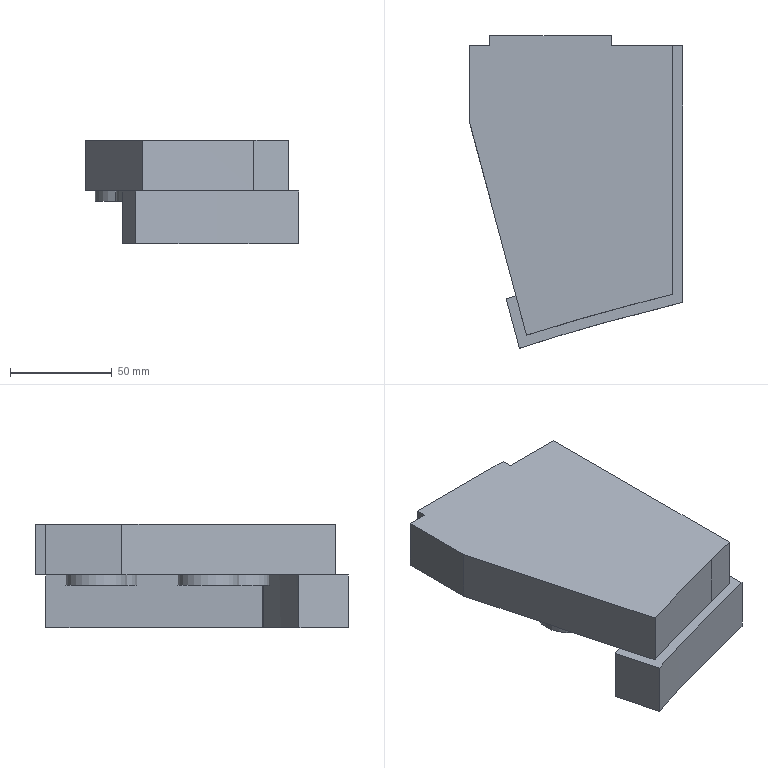Part | NX | features solid 2 | 1 solid | 29 faces | box 104.575 x 153.355 x 51 mm | volume 442885 mm3 | plane 20 | spline 5 | cylinder 4 | commonest cylinder face diameters 30 x4
STEP:
#1=CARTESIAN_POINT('',(-394.575,600.,45.));
#2=VERTEX_POINT('',#1);
#3=CARTESIAN_POINT('',(-394.575,600.,20.));
#4=VERTEX_POINT('',#3);
#5=CARTESIAN_POINT('',(-394.575,600.,50.));
#6=DIRECTION('',(0.,0.,-1.));
#7=VECTOR('',#6,1000.);
#8=LINE('',#5,#7);
#9=EDGE_CURVE('',#2,#4,#8,.T.);
#10=ORIENTED_EDGE('',*,*,#9,.F.);
#11=CARTESIAN_POINT('',(-384.575,600.,45.));
#12=VERTEX_POINT('',#11);
#13=CARTESIAN_POINT('',(-290.,600.,45.));
#14=DIRECTION('',(-1.,0.,0.));
#15=VECTOR('',#14,1000.);
#16=LINE('',#13,#15);
#17=EDGE_CURVE('',#12,#2,#16,.T.);
#18=ORIENTED_EDGE('',*,*,#17,.F.);
#19=CARTESIAN_POINT('',(-384.575,600.,20.));
#20=VERTEX_POINT('',#19);
#21=CARTESIAN_POINT('',(-384.575,600.,50.));
#22=DIRECTION('',(0.,0.,-1.));
#23=VECTOR('',#22,1000.);
#24=LINE('',#21,#23);
#25=EDGE_CURVE('',#12,#20,#24,.T.);
#26=ORIENTED_EDGE('',*,*,#25,.T.);
#27=CARTESIAN_POINT('',(-561.977,600.,20.));
#28=DIRECTION('',(1.,0.,0.));
#29=VECTOR('',#28,1000.);
#30=LINE('',#27,#29);
#31=EDGE_CURVE('',#20,#4,#30,.F.);
#32=ORIENTED_EDGE('',*,*,#31,.T.);
#33=EDGE_LOOP('',(#10,#18,#26,#32));
#34=FACE_BOUND('',#33,.T.);
#35=CARTESIAN_POINT('',(-290.,600.,50.));
#36=DIRECTION('',(0.,-1.,0.));
#37=DIRECTION('',(0.,0.,-1.));
#38=AXIS2_PLACEMENT_3D('',#35,#36,#37);
#39=PLANE('',#38);
#40=ADVANCED_FACE('',(#34),#39,.F.);
#41=ORIENTED_EDGE('',*,*,#17,.T.);
#42=CARTESIAN_POINT('',(-394.575,562.679,45.));
#43=VERTEX_POINT('',#42);
#44=CARTESIAN_POINT('',(-394.575,-794.984,45.));
#45=DIRECTION('',(0.,-1.,0.));
#46=VECTOR('',#45,1000.);
#47=LINE('',#44,#46);
#48=EDGE_CURVE('',#2,#43,#47,.T.);
#49=ORIENTED_EDGE('',*,*,#48,.T.);
#50=CARTESIAN_POINT('',(-366.532,458.021,45.));
#51=VERTEX_POINT('',#50);
#52=CARTESIAN_POINT('',(-371.65,477.121,45.));
#53=DIRECTION('',(-0.2588,0.9659,0.));
#54=VECTOR('',#53,1000.);
#55=LINE('',#52,#54);
#56=EDGE_CURVE('',#43,#51,#55,.F.);
#57=ORIENTED_EDGE('',*,*,#56,.T.);
#58=CARTESIAN_POINT('',(-311.881,473.776,45.));
#59=VERTEX_POINT('',#58);
#60=CARTESIAN_POINT('',(-366.532,458.021,45.));
#61=CARTESIAN_POINT('',(-361.995,459.474,45.));
#62=CARTESIAN_POINT('',(-355.189,461.6,45.));
#63=CARTESIAN_POINT('',(-347.268,463.978,45.));
#64=CARTESIAN_POINT('',(-343.294,465.147,45.));
#65=CARTESIAN_POINT('',(-341.047,465.801,45.));
#66=CARTESIAN_POINT('',(-339.295,466.308,45.));
#67=CARTESIAN_POINT('',(-337.801,466.736,45.));
#68=CARTESIAN_POINT('',(-335.683,467.34,45.));
#69=CARTESIAN_POINT('',(-331.945,468.393,45.));
#70=CARTESIAN_POINT('',(-326.364,469.934,45.));
#71=CARTESIAN_POINT('',(-319.327,471.827,45.));
#72=CARTESIAN_POINT('',(-314.402,473.121,45.));
#73=CARTESIAN_POINT('',(-311.881,473.776,45.));
#74=B_SPLINE_CURVE_WITH_KNOTS('',3,(#60,#61,#62,#63,#64,#65,#66,#67,#68,#69,#70,#71,#72,#73),.UNSPECIFIED.,.F.,.F.,(4,1,1,1,1,1,1,1,1,1,1,4),(0.,0.25,0.375,0.4375,0.4688,0.5,0.5312,0.5625,0.625,0.75,0.875,1.),.UNSPECIFIED.);
#75=EDGE_CURVE('',#51,#59,#74,.T.);
#76=ORIENTED_EDGE('',*,*,#75,.T.);
#77=CARTESIAN_POINT('',(-295.,478.098,45.));
#78=VERTEX_POINT('',#77);
#79=CARTESIAN_POINT('',(-311.881,473.776,45.));
#80=CARTESIAN_POINT('',(-307.372,474.947,45.));
#81=CARTESIAN_POINT('',(-301.745,476.387,45.));
#82=CARTESIAN_POINT('',(-295.,478.098,45.));
#83=B_SPLINE_CURVE_WITH_KNOTS('',3,(#79,#80,#81,#82),.UNSPECIFIED.,.F.,.F.,(4,4),(0.,1.),.UNSPECIFIED.);
#84=EDGE_CURVE('',#59,#78,#83,.T.);
#85=ORIENTED_EDGE('',*,*,#84,.T.);
#86=CARTESIAN_POINT('',(-295.,600.,45.));
#87=VERTEX_POINT('',#86);
#88=CARTESIAN_POINT('',(-295.,-794.984,45.));
#89=DIRECTION('',(0.,1.,0.));
#90=VECTOR('',#89,1000.);
#91=LINE('',#88,#90);
#92=EDGE_CURVE('',#78,#87,#91,.T.);
#93=ORIENTED_EDGE('',*,*,#92,.T.);
#94=CARTESIAN_POINT('',(-325.,600.,45.));
#95=VERTEX_POINT('',#94);
#96=CARTESIAN_POINT('',(-290.,600.,45.));
#97=DIRECTION('',(-1.,0.,0.));
#98=VECTOR('',#97,1000.);
#99=LINE('',#96,#98);
#100=EDGE_CURVE('',#87,#95,#99,.T.);
#101=ORIENTED_EDGE('',*,*,#100,.T.);
#102=CARTESIAN_POINT('',(-325.,605.,45.));
#103=VERTEX_POINT('',#102);
#104=CARTESIAN_POINT('',(-325.,605.,45.));
#105=DIRECTION('',(0.,-1.,0.));
#106=VECTOR('',#105,1000.);
#107=LINE('',#104,#106);
#108=EDGE_CURVE('',#103,#95,#107,.T.);
#109=ORIENTED_EDGE('',*,*,#108,.F.);
#110=CARTESIAN_POINT('',(-384.575,605.,45.));
#111=VERTEX_POINT('',#110);
#112=CARTESIAN_POINT('',(-290.,605.,45.));
#113=DIRECTION('',(-1.,0.,0.));
#114=VECTOR('',#113,1000.);
#115=LINE('',#112,#114);
#116=EDGE_CURVE('',#103,#111,#115,.T.);
#117=ORIENTED_EDGE('',*,*,#116,.T.);
#118=CARTESIAN_POINT('',(-384.575,605.,45.));
#119=DIRECTION('',(0.,-1.,0.));
#120=VECTOR('',#119,1000.);
#121=LINE('',#118,#120);
#122=EDGE_CURVE('',#111,#12,#121,.T.);
#123=ORIENTED_EDGE('',*,*,#122,.T.);
#124=EDGE_LOOP('',(#41,#49,#57,#76,#85,#93,#101,#109,#117,#123));
#125=FACE_BOUND('',#124,.T.);
#126=CARTESIAN_POINT('',(-80.139,-794.984,45.));
#127=DIRECTION('',(0.,0.,1.));
#128=DIRECTION('',(1.,0.,0.));
#129=AXIS2_PLACEMENT_3D('',#126,#127,#128);
#130=PLANE('',#129);
#131=ADVANCED_FACE('',(#125),#130,.T.);
#132=CARTESIAN_POINT('',(-354.757,570.324,20.));
#133=VERTEX_POINT('',#132);
#134=CARTESIAN_POINT('',(-339.757,570.324,20.));
#135=DIRECTION('',(0.,0.,-1.));
#136=DIRECTION('',(-1.,0.,0.));
#137=AXIS2_PLACEMENT_3D('',#134,#135,#136);
#138=CIRCLE('',#137,15.);
#139=EDGE_CURVE('',#133,#133,#138,.F.);
#140=ORIENTED_EDGE('',*,*,#139,.T.);
#141=EDGE_LOOP('',(#140));
#142=FACE_BOUND('',#141,.T.);
#143=CARTESIAN_POINT('',(-389.757,575.324,20.));
#144=VERTEX_POINT('',#143);
#145=CARTESIAN_POINT('',(-374.757,575.324,20.));
#146=DIRECTION('',(0.,0.,-1.));
#147=DIRECTION('',(-1.,0.,0.));
#148=AXIS2_PLACEMENT_3D('',#145,#146,#147);
#149=CIRCLE('',#148,15.);
#150=EDGE_CURVE('',#144,#144,#149,.F.);
#151=ORIENTED_EDGE('',*,*,#150,.T.);
#152=EDGE_LOOP('',(#151));
#153=FACE_BOUND('',#152,.T.);
#154=CARTESIAN_POINT('',(-349.757,505.324,20.));
#155=VERTEX_POINT('',#154);
#156=CARTESIAN_POINT('',(-334.757,505.324,20.));
#157=DIRECTION('',(0.,0.,-1.));
#158=DIRECTION('',(-1.,0.,0.));
#159=AXIS2_PLACEMENT_3D('',#156,#157,#158);
#160=CIRCLE('',#159,15.);
#161=EDGE_CURVE('',#155,#155,#160,.F.);
#162=ORIENTED_EDGE('',*,*,#161,.T.);
#163=EDGE_LOOP('',(#162));
#164=FACE_BOUND('',#163,.T.);
#165=CARTESIAN_POINT('',(-379.757,520.324,20.));
#166=VERTEX_POINT('',#165);
#167=CARTESIAN_POINT('',(-364.757,520.324,20.));
#168=DIRECTION('',(0.,0.,-1.));
#169=DIRECTION('',(-1.,0.,0.));
#170=AXIS2_PLACEMENT_3D('',#167,#168,#169);
#171=CIRCLE('',#170,15.);
#172=EDGE_CURVE('',#166,#166,#171,.F.);
#173=ORIENTED_EDGE('',*,*,#172,.T.);
#174=EDGE_LOOP('',(#173));
#175=FACE_BOUND('',#174,.T.);
#176=CARTESIAN_POINT('',(-394.575,562.679,20.));
#177=VERTEX_POINT('',#176);
#178=CARTESIAN_POINT('',(-394.575,359.461,20.));
#179=DIRECTION('',(0.,1.,0.));
#180=VECTOR('',#179,1000.);
#181=LINE('',#178,#180);
#182=EDGE_CURVE('',#4,#177,#181,.F.);
#183=ORIENTED_EDGE('',*,*,#182,.F.);
#184=ORIENTED_EDGE('',*,*,#31,.F.);
#185=CARTESIAN_POINT('',(-384.575,605.,20.));
#186=VERTEX_POINT('',#185);
#187=CARTESIAN_POINT('',(-384.575,605.,20.));
#188=DIRECTION('',(0.,-1.,0.));
#189=VECTOR('',#188,1000.);
#190=LINE('',#187,#189);
#191=EDGE_CURVE('',#186,#20,#190,.T.);
#192=ORIENTED_EDGE('',*,*,#191,.F.);
#193=CARTESIAN_POINT('',(-325.,605.,20.));
#194=VERTEX_POINT('',#193);
#195=CARTESIAN_POINT('',(-561.977,605.,20.));
#196=DIRECTION('',(1.,0.,0.));
#197=VECTOR('',#196,1000.);
#198=LINE('',#195,#197);
#199=EDGE_CURVE('',#194,#186,#198,.F.);
#200=ORIENTED_EDGE('',*,*,#199,.F.);
#201=CARTESIAN_POINT('',(-325.,600.,20.));
#202=VERTEX_POINT('',#201);
#203=CARTESIAN_POINT('',(-325.,605.,20.));
#204=DIRECTION('',(0.,-1.,0.));
#205=VECTOR('',#204,1000.);
#206=LINE('',#203,#205);
#207=EDGE_CURVE('',#194,#202,#206,.T.);
#208=ORIENTED_EDGE('',*,*,#207,.T.);
#209=CARTESIAN_POINT('',(-315.,600.,20.));
#210=VERTEX_POINT('',#209);
#211=CARTESIAN_POINT('',(-561.977,600.,20.));
#212=DIRECTION('',(1.,0.,0.));
#213=VECTOR('',#212,1000.);
#214=LINE('',#211,#213);
#215=EDGE_CURVE('',#210,#202,#214,.F.);
#216=ORIENTED_EDGE('',*,*,#215,.F.);
#217=CARTESIAN_POINT('',(-315.,493.628,20.));
#218=VERTEX_POINT('',#217);
#219=CARTESIAN_POINT('',(-315.,359.461,20.));
#220=DIRECTION('',(0.,1.,0.));
#221=VECTOR('',#220,1000.);
#222=LINE('',#219,#221);
#223=EDGE_CURVE('',#210,#218,#222,.F.);
#224=ORIENTED_EDGE('',*,*,#223,.T.);
#225=CARTESIAN_POINT('',(-316.72,493.182,20.));
#226=VERTEX_POINT('',#225);
#227=CARTESIAN_POINT('',(-316.72,493.182,20.));
#228=CARTESIAN_POINT('',(-316.146,493.331,20.));
#229=CARTESIAN_POINT('',(-315.573,493.48,20.));
#230=CARTESIAN_POINT('',(-315.,493.628,20.));
#231=B_SPLINE_CURVE_WITH_KNOTS('',3,(#227,#228,#229,#230),.UNSPECIFIED.,.F.,.F.,(4,4),(0.4269,0.4287),.UNSPECIFIED.);
#232=EDGE_CURVE('',#226,#218,#231,.T.);
#233=ORIENTED_EDGE('',*,*,#232,.F.);
#234=CARTESIAN_POINT('',(-371.714,477.362,20.));
#235=VERTEX_POINT('',#234);
#236=CARTESIAN_POINT('',(-371.714,477.362,20.));
#237=CARTESIAN_POINT('',(-353.545,483.162,20.));
#238=CARTESIAN_POINT('',(-335.183,488.388,20.));
#239=CARTESIAN_POINT('',(-316.72,493.182,20.));
#240=B_SPLINE_CURVE_WITH_KNOTS('',3,(#236,#237,#238,#239),.UNSPECIFIED.,.F.,.F.,(4,4),(0.6725,0.7298),.UNSPECIFIED.);
#241=EDGE_CURVE('',#235,#226,#240,.T.);
#242=ORIENTED_EDGE('',*,*,#241,.F.);
#243=CARTESIAN_POINT('',(-371.65,477.121,20.));
#244=DIRECTION('',(0.2588,-0.9659,0.));
#245=VECTOR('',#244,1000.);
#246=LINE('',#243,#245);
#247=EDGE_CURVE('',#177,#235,#246,.T.);
#248=ORIENTED_EDGE('',*,*,#247,.F.);
#249=EDGE_LOOP('',(#183,#184,#192,#200,#208,#216,#224,#233,#242,#248));
#250=FACE_BOUND('',#249,.T.);
#251=CARTESIAN_POINT('',(-561.977,359.461,20.));
#252=DIRECTION('',(0.,0.,-1.));
#253=DIRECTION('',(-1.,0.,0.));
#254=AXIS2_PLACEMENT_3D('',#251,#252,#253);
#255=PLANE('',#254);
#256=ADVANCED_FACE('',(#142,#153,#164,#175,#250),#255,.T.);
#257=ORIENTED_EDGE('',*,*,#56,.F.);
#258=CARTESIAN_POINT('',(-394.575,562.679,20.));
#259=DIRECTION('',(0.,0.,-1.));
#260=VECTOR('',#259,1000.);
#261=LINE('',#258,#260);
#262=EDGE_CURVE('',#43,#177,#261,.T.);
#263=ORIENTED_EDGE('',*,*,#262,.T.);
#264=ORIENTED_EDGE('',*,*,#247,.T.);
#265=CARTESIAN_POINT('',(-366.532,458.021,20.));
#266=VERTEX_POINT('',#265);
#267=CARTESIAN_POINT('',(-371.65,477.121,20.));
#268=DIRECTION('',(0.2588,-0.9659,0.));
#269=VECTOR('',#268,1000.);
#270=LINE('',#267,#269);
#271=EDGE_CURVE('',#235,#266,#270,.T.);
#272=ORIENTED_EDGE('',*,*,#271,.T.);
#273=CARTESIAN_POINT('',(-366.532,458.021,32.5));
#274=DIRECTION('',(0.,0.,-1.));
#275=VECTOR('',#274,1000.);
#276=LINE('',#273,#275);
#277=EDGE_CURVE('',#266,#51,#276,.F.);
#278=ORIENTED_EDGE('',*,*,#277,.T.);
#279=EDGE_LOOP('',(#257,#263,#264,#272,#278));
#280=FACE_BOUND('',#279,.T.);
#281=CARTESIAN_POINT('',(-371.65,477.121,20.));
#282=DIRECTION('',(-0.9659,-0.2588,0.));
#283=DIRECTION('',(0.2588,-0.9659,0.));
#284=AXIS2_PLACEMENT_3D('',#281,#282,#283);
#285=PLANE('',#284);
#286=ADVANCED_FACE('',(#280),#285,.T.);
#287=ORIENTED_EDGE('',*,*,#277,.F.);
#288=CARTESIAN_POINT('',(-311.881,473.776,20.));
#289=VERTEX_POINT('',#288);
#290=CARTESIAN_POINT('',(-366.532,458.021,20.));
#291=CARTESIAN_POINT('',(-348.472,463.806,20.));
#292=CARTESIAN_POINT('',(-330.24,469.008,20.));
#293=CARTESIAN_POINT('',(-311.881,473.776,20.));
#294=B_SPLINE_CURVE_WITH_KNOTS('',3,(#290,#291,#292,#293),.UNSPECIFIED.,.F.,.F.,(4,4),(1.334,1.391),.UNSPECIFIED.);
#295=EDGE_CURVE('',#266,#289,#294,.T.);
#296=ORIENTED_EDGE('',*,*,#295,.T.);
#297=CARTESIAN_POINT('',(-311.881,473.776,32.5));
#298=DIRECTION('',(0.,0.,-1.));
#299=VECTOR('',#298,1000.);
#300=LINE('',#297,#299);
#301=EDGE_CURVE('',#59,#289,#300,.T.);
#302=ORIENTED_EDGE('',*,*,#301,.F.);
#303=ORIENTED_EDGE('',*,*,#75,.F.);
#304=EDGE_LOOP('',(#287,#296,#302,#303));
#305=FACE_BOUND('',#304,.T.);
#306=CARTESIAN_POINT('',(-366.532,458.021,45.));
#307=CARTESIAN_POINT('',(-366.532,458.021,20.));
#308=CARTESIAN_POINT('',(-357.499,460.914,45.));
#309=CARTESIAN_POINT('',(-357.499,460.914,20.));
#310=CARTESIAN_POINT('',(-339.371,466.444,45.));
#311=CARTESIAN_POINT('',(-339.371,466.444,20.));
#312=CARTESIAN_POINT('',(-321.012,471.404,45.));
#313=CARTESIAN_POINT('',(-321.012,471.404,20.));
#314=CARTESIAN_POINT('',(-311.881,473.776,45.));
#315=CARTESIAN_POINT('',(-311.881,473.776,20.));
#316=B_SPLINE_SURFACE_WITH_KNOTS('',3,1,((#306,#307),(#308,#309),(#310,#311),(#312,#313),(#314,#315)),.SURF_OF_LINEAR_EXTRUSION.,.F.,.F.,.F.,(4,1,4),(2,2),(0.7947,0.8974,1.),(0.,1.),.UNSPECIFIED.);
#317=ADVANCED_FACE('',(#305),#316,.F.);
#318=ORIENTED_EDGE('',*,*,#215,.T.);
#319=CARTESIAN_POINT('',(-325.,600.,50.));
#320=DIRECTION('',(0.,0.,1.));
#321=VECTOR('',#320,1000.);
#322=LINE('',#319,#321);
#323=EDGE_CURVE('',#202,#95,#322,.T.);
#324=ORIENTED_EDGE('',*,*,#323,.T.);
#325=ORIENTED_EDGE('',*,*,#100,.F.);
#326=CARTESIAN_POINT('',(-295.,600.,20.));
#327=VERTEX_POINT('',#326);
#328=CARTESIAN_POINT('',(-295.,600.,50.));
#329=DIRECTION('',(0.,0.,1.));
#330=VECTOR('',#329,1000.);
#331=LINE('',#328,#330);
#332=EDGE_CURVE('',#327,#87,#331,.T.);
#333=ORIENTED_EDGE('',*,*,#332,.F.);
#334=CARTESIAN_POINT('',(-290.,600.,20.));
#335=VERTEX_POINT('',#334);
#336=CARTESIAN_POINT('',(-290.,600.,20.));
#337=DIRECTION('',(1.,0.,0.));
#338=VECTOR('',#337,1000.);
#339=LINE('',#336,#338);
#340=EDGE_CURVE('',#335,#327,#339,.F.);
#341=ORIENTED_EDGE('',*,*,#340,.F.);
#342=CARTESIAN_POINT('',(-290.,600.,-6.));
#343=VERTEX_POINT('',#342);
#344=CARTESIAN_POINT('',(-290.,600.,50.));
#345=DIRECTION('',(0.,0.,-1.));
#346=VECTOR('',#345,1000.);
#347=LINE('',#344,#346);
#348=EDGE_CURVE('',#335,#343,#347,.T.);
#349=ORIENTED_EDGE('',*,*,#348,.T.);
#350=CARTESIAN_POINT('',(-315.,600.,-6.));
#351=VERTEX_POINT('',#350);
#352=CARTESIAN_POINT('',(-290.,600.,-6.));
#353=DIRECTION('',(-1.,0.,0.));
#354=VECTOR('',#353,1000.);
#355=LINE('',#352,#354);
#356=EDGE_CURVE('',#343,#351,#355,.T.);
#357=ORIENTED_EDGE('',*,*,#356,.T.);
#358=CARTESIAN_POINT('',(-315.,600.,50.));
#359=DIRECTION('',(0.,0.,-1.));
#360=VECTOR('',#359,1000.);
#361=LINE('',#358,#360);
#362=EDGE_CURVE('',#210,#351,#361,.T.);
#363=ORIENTED_EDGE('',*,*,#362,.F.);
#364=EDGE_LOOP('',(#318,#324,#325,#333,#341,#349,#357,#363));
#365=FACE_BOUND('',#364,.T.);
#366=CARTESIAN_POINT('',(-290.,600.,50.));
#367=DIRECTION('',(0.,-1.,0.));
#368=DIRECTION('',(0.,0.,-1.));
#369=AXIS2_PLACEMENT_3D('',#366,#367,#368);
#370=PLANE('',#369);
#371=ADVANCED_FACE('',(#365),#370,.F.);
#372=ORIENTED_EDGE('',*,*,#223,.F.);
#373=ORIENTED_EDGE('',*,*,#362,.T.);
#374=CARTESIAN_POINT('',(-315.,493.628,-6.));
#375=VERTEX_POINT('',#374);
#376=CARTESIAN_POINT('',(-315.,467.794,-6.));
#377=DIRECTION('',(0.,1.,0.));
#378=VECTOR('',#377,1000.);
#379=LINE('',#376,#378);
#380=EDGE_CURVE('',#375,#351,#379,.T.);
#381=ORIENTED_EDGE('',*,*,#380,.F.);
#382=CARTESIAN_POINT('',(-315.,493.628,7.));
#383=DIRECTION('',(0.,0.,1.));
#384=VECTOR('',#383,1000.);
#385=LINE('',#382,#384);
#386=EDGE_CURVE('',#218,#375,#385,.F.);
#387=ORIENTED_EDGE('',*,*,#386,.F.);
#388=EDGE_LOOP('',(#372,#373,#381,#387));
#389=FACE_BOUND('',#388,.T.);
#390=CARTESIAN_POINT('',(-315.,467.794,50.));
#391=DIRECTION('',(-1.,0.,0.));
#392=DIRECTION('',(0.,0.,1.));
#393=AXIS2_PLACEMENT_3D('',#390,#391,#392);
#394=PLANE('',#393);
#395=ADVANCED_FACE('',(#389),#394,.T.);
#396=CARTESIAN_POINT('',(-295.,478.098,20.));
#397=VERTEX_POINT('',#396);
#398=CARTESIAN_POINT('',(-295.,478.098,32.5));
#399=DIRECTION('',(0.,0.,-1.));
#400=VECTOR('',#399,1000.);
#401=LINE('',#398,#400);
#402=EDGE_CURVE('',#78,#397,#401,.T.);
#403=ORIENTED_EDGE('',*,*,#402,.F.);
#404=ORIENTED_EDGE('',*,*,#84,.F.);
#405=ORIENTED_EDGE('',*,*,#301,.T.);
#406=CARTESIAN_POINT('',(-311.881,473.776,20.));
#407=CARTESIAN_POINT('',(-306.259,475.236,20.));
#408=CARTESIAN_POINT('',(-300.63,476.67,20.));
#409=CARTESIAN_POINT('',(-295.,478.098,20.));
#410=B_SPLINE_CURVE_WITH_KNOTS('',3,(#406,#407,#408,#409),.UNSPECIFIED.,.F.,.F.,(4,4),(1.091,1.108),.UNSPECIFIED.);
#411=EDGE_CURVE('',#289,#397,#410,.T.);
#412=ORIENTED_EDGE('',*,*,#411,.T.);
#413=EDGE_LOOP('',(#403,#404,#405,#412));
#414=FACE_BOUND('',#413,.T.);
#415=CARTESIAN_POINT('',(-311.881,473.776,45.));
#416=CARTESIAN_POINT('',(-311.881,473.776,20.));
#417=CARTESIAN_POINT('',(-306.253,475.237,45.));
#418=CARTESIAN_POINT('',(-306.253,475.237,20.));
#419=CARTESIAN_POINT('',(-300.625,476.671,45.));
#420=CARTESIAN_POINT('',(-300.625,476.671,20.));
#421=CARTESIAN_POINT('',(-295.,478.098,45.));
#422=CARTESIAN_POINT('',(-295.,478.098,20.));
#423=B_SPLINE_SURFACE_WITH_KNOTS('',3,1,((#415,#416),(#417,#418),(#419,#420),(#421,#422)),.SURF_OF_LINEAR_EXTRUSION.,.F.,.F.,.F.,(4,4),(2,2),(0.0001799,0.06461),(0.,1.),.PIECEWISE_BEZIER_KNOTS.);
#424=ADVANCED_FACE('',(#414),#423,.F.);
#425=ORIENTED_EDGE('',*,*,#348,.F.);
#426=CARTESIAN_POINT('',(-290.,474.207,20.));
#427=VERTEX_POINT('',#426);
#428=CARTESIAN_POINT('',(-290.,359.461,20.));
#429=DIRECTION('',(0.,-1.,0.));
#430=VECTOR('',#429,1000.);
#431=LINE('',#428,#430);
#432=EDGE_CURVE('',#427,#335,#431,.F.);
#433=ORIENTED_EDGE('',*,*,#432,.F.);
#434=CARTESIAN_POINT('',(-290.,474.207,-6.));
#435=VERTEX_POINT('',#434);
#436=CARTESIAN_POINT('',(-290.,474.207,7.));
#437=DIRECTION('',(0.,0.,-1.));
#438=VECTOR('',#437,1000.);
#439=LINE('',#436,#438);
#440=EDGE_CURVE('',#435,#427,#439,.F.);
#441=ORIENTED_EDGE('',*,*,#440,.F.);
#442=CARTESIAN_POINT('',(-290.,-794.984,-6.));
#443=DIRECTION('',(0.,-1.,0.));
#444=VECTOR('',#443,1000.);
#445=LINE('',#442,#444);
#446=EDGE_CURVE('',#343,#435,#445,.T.);
#447=ORIENTED_EDGE('',*,*,#446,.F.);
#448=EDGE_LOOP('',(#425,#433,#441,#447));
#449=FACE_BOUND('',#448,.T.);
#450=CARTESIAN_POINT('',(-290.,600.,0.));
#451=DIRECTION('',(-1.,0.,0.));
#452=DIRECTION('',(0.,0.,1.));
#453=AXIS2_PLACEMENT_3D('',#450,#451,#452);
#454=PLANE('',#453);
#455=ADVANCED_FACE('',(#449),#454,.F.);
#456=CARTESIAN_POINT('',(-376.48,475.827,20.));
#457=VERTEX_POINT('',#456);
#458=CARTESIAN_POINT('',(-376.48,475.827,-6.));
#459=VERTEX_POINT('',#458);
#460=CARTESIAN_POINT('',(-376.48,475.827,7.));
#461=DIRECTION('',(0.,0.,1.));
#462=VECTOR('',#461,1000.);
#463=LINE('',#460,#462);
#464=EDGE_CURVE('',#457,#459,#463,.F.);
#465=ORIENTED_EDGE('',*,*,#464,.F.);
#466=CARTESIAN_POINT('',(-376.48,475.827,20.));
#467=CARTESIAN_POINT('',(-374.893,476.342,20.));
#468=CARTESIAN_POINT('',(-373.304,476.854,20.));
#469=CARTESIAN_POINT('',(-371.714,477.362,20.));
#470=B_SPLINE_CURVE_WITH_KNOTS('',3,(#466,#467,#468,#469),.UNSPECIFIED.,.F.,.F.,(4,4),(0.6675,0.6725),.UNSPECIFIED.);
#471=EDGE_CURVE('',#457,#235,#470,.T.);
#472=ORIENTED_EDGE('',*,*,#471,.T.);
#473=ORIENTED_EDGE('',*,*,#241,.T.);
#474=CARTESIAN_POINT('',(-316.72,493.182,-6.));
#475=VERTEX_POINT('',#474);
#476=CARTESIAN_POINT('',(-316.72,493.182,9.5));
#477=DIRECTION('',(0.,0.,1.));
#478=VECTOR('',#477,1000.);
#479=LINE('',#476,#478);
#480=EDGE_CURVE('',#475,#226,#479,.T.);
#481=ORIENTED_EDGE('',*,*,#480,.F.);
#482=CARTESIAN_POINT('',(-376.48,475.827,-6.));
#483=CARTESIAN_POINT('',(-356.756,482.235,-6.));
#484=CARTESIAN_POINT('',(-336.798,487.968,-6.));
#485=CARTESIAN_POINT('',(-316.72,493.182,-6.));
#486=B_SPLINE_CURVE_WITH_KNOTS('',3,(#482,#483,#484,#485),.UNSPECIFIED.,.F.,.F.,(4,4),(0.6679,0.7302),.UNSPECIFIED.);
#487=EDGE_CURVE('',#459,#475,#486,.T.);
#488=ORIENTED_EDGE('',*,*,#487,.F.);
#489=EDGE_LOOP('',(#465,#472,#473,#481,#488));
#490=FACE_BOUND('',#489,.T.);
#491=CARTESIAN_POINT('',(-376.48,475.827,-6.));
#492=CARTESIAN_POINT('',(-376.48,475.827,20.));
#493=CARTESIAN_POINT('',(-366.597,479.038,-6.));
#494=CARTESIAN_POINT('',(-366.597,479.038,20.));
#495=CARTESIAN_POINT('',(-351.726,483.613,-6.));
#496=CARTESIAN_POINT('',(-351.726,483.613,20.));
#497=CARTESIAN_POINT('',(-334.183,488.552,-6.));
#498=CARTESIAN_POINT('',(-334.183,488.552,20.));
#499=CARTESIAN_POINT('',(-324.189,491.233,-6.));
#500=CARTESIAN_POINT('',(-324.189,491.233,20.));
#501=CARTESIAN_POINT('',(-319.169,492.546,-6.));
#502=CARTESIAN_POINT('',(-319.169,492.546,20.));
#503=CARTESIAN_POINT('',(-316.72,493.182,-6.));
#504=CARTESIAN_POINT('',(-316.72,493.182,20.));
#505=B_SPLINE_SURFACE_WITH_KNOTS('',3,1,((#491,#492),(#493,#494),(#495,#496),(#497,#498),(#499,#500),(#501,#502),(#503,#504)),.SURF_OF_LINEAR_EXTRUSION.,.F.,.F.,.F.,(4,1,1,1,4),(2,2),(0.7804,0.8906,0.9458,0.9733,1.001),(0.,1.),.UNSPECIFIED.);
#506=ADVANCED_FACE('',(#490),#505,.F.);
#507=CARTESIAN_POINT('',(-370.,451.645,20.));
#508=VERTEX_POINT('',#507);
#509=CARTESIAN_POINT('',(-359.814,413.63,20.));
#510=DIRECTION('',(0.2588,-0.9659,0.));
#511=VECTOR('',#510,1000.);
#512=LINE('',#509,#511);
#513=EDGE_CURVE('',#508,#457,#512,.F.);
#514=ORIENTED_EDGE('',*,*,#513,.T.);
#515=ORIENTED_EDGE('',*,*,#464,.T.);
#516=CARTESIAN_POINT('',(-370.,451.645,-6.));
#517=VERTEX_POINT('',#516);
#518=CARTESIAN_POINT('',(-38.926,-783.941,-6.));
#519=DIRECTION('',(0.2588,-0.9659,0.));
#520=VECTOR('',#519,1000.);
#521=LINE('',#518,#520);
#522=EDGE_CURVE('',#459,#517,#521,.T.);
#523=ORIENTED_EDGE('',*,*,#522,.T.);
#524=CARTESIAN_POINT('',(-370.,451.645,7.));
#525=DIRECTION('',(0.,0.,-1.));
#526=VECTOR('',#525,1000.);
#527=LINE('',#524,#526);
#528=EDGE_CURVE('',#517,#508,#527,.F.);
#529=ORIENTED_EDGE('',*,*,#528,.T.);
#530=EDGE_LOOP('',(#514,#515,#523,#529));
#531=FACE_BOUND('',#530,.T.);
#532=CARTESIAN_POINT('',(-409.752,600.,0.));
#533=DIRECTION('',(-0.9659,-0.2588,0.));
#534=DIRECTION('',(0.2588,-0.9659,0.));
#535=AXIS2_PLACEMENT_3D('',#532,#533,#534);
#536=PLANE('',#535);
#537=ADVANCED_FACE('',(#531),#536,.T.);
#538=CARTESIAN_POINT('',(-316.72,493.182,-6.));
#539=VERTEX_POINT('',#538);
#540=CARTESIAN_POINT('',(-316.72,493.182,9.5));
#541=DIRECTION('',(0.,0.,1.));
#542=VECTOR('',#541,1000.);
#543=LINE('',#540,#542);
#544=EDGE_CURVE('',#539,#226,#543,.T.);
#545=ORIENTED_EDGE('',*,*,#544,.F.);
#546=CARTESIAN_POINT('',(301.428,-1986.073,-6.));
#547=DIRECTION('',(-0.2419,0.9703,0.));
#548=VECTOR('',#547,1000.);
#549=LINE('',#546,#548);
#550=EDGE_CURVE('',#539,#475,#549,.T.);
#551=ORIENTED_EDGE('',*,*,#550,.T.);
#552=ORIENTED_EDGE('',*,*,#480,.T.);
#553=EDGE_LOOP('',(#545,#551,#552));
#554=FACE_BOUND('',#553,.T.);
#555=CARTESIAN_POINT('',(301.428,-1986.073,70.));
#556=DIRECTION('',(-0.9703,-0.2419,0.));
#557=DIRECTION('',(0.2419,-0.9703,0.));
#558=AXIS2_PLACEMENT_3D('',#555,#556,#557);
#559=PLANE('',#558);
#560=ADVANCED_FACE('',(#554),#559,.F.);
#561=CARTESIAN_POINT('',(-290.,474.207,20.));
#562=CARTESIAN_POINT('',(-303.431,470.806,20.));
#563=CARTESIAN_POINT('',(-330.29,463.995,20.));
#564=CARTESIAN_POINT('',(-356.814,455.949,20.));
#565=CARTESIAN_POINT('',(-370.,451.645,20.));
#566=B_SPLINE_CURVE_WITH_KNOTS('',3,(#561,#562,#563,#564,#565),.UNSPECIFIED.,.F.,.F.,(4,1,4),(0.7156,0.7571,0.7987),.UNSPECIFIED.);
#567=EDGE_CURVE('',#508,#427,#566,.F.);
#568=ORIENTED_EDGE('',*,*,#567,.T.);
#569=ORIENTED_EDGE('',*,*,#432,.T.);
#570=ORIENTED_EDGE('',*,*,#340,.T.);
#571=CARTESIAN_POINT('',(-295.,482.459,20.));
#572=DIRECTION('',(0.,1.,0.));
#573=VECTOR('',#572,1000.);
#574=LINE('',#571,#573);
#575=EDGE_CURVE('',#397,#327,#574,.T.);
#576=ORIENTED_EDGE('',*,*,#575,.F.);
#577=ORIENTED_EDGE('',*,*,#411,.F.);
#578=CARTESIAN_POINT('',(-316.7,472.438,20.));
#579=VERTEX_POINT('',#578);
#580=CARTESIAN_POINT('',(-311.881,473.776,20.));
#581=CARTESIAN_POINT('',(-313.487,473.33,20.));
#582=CARTESIAN_POINT('',(-315.094,472.884,20.));
#583=CARTESIAN_POINT('',(-316.7,472.438,20.));
#584=B_SPLINE_CURVE_WITH_KNOTS('',3,(#580,#581,#582,#583),.UNSPECIFIED.,.F.,.F.,(4,4),(0.,0.1323),.UNSPECIFIED.);
#585=EDGE_CURVE('',#289,#579,#584,.T.);
#586=ORIENTED_EDGE('',*,*,#585,.T.);
#587=ORIENTED_EDGE('',*,*,#585,.F.);
#588=ORIENTED_EDGE('',*,*,#295,.F.);
#589=ORIENTED_EDGE('',*,*,#271,.F.);
#590=ORIENTED_EDGE('',*,*,#471,.F.);
#591=ORIENTED_EDGE('',*,*,#513,.F.);
#592=EDGE_LOOP('',(#568,#569,#570,#576,#577,#586,#587,#588,#589,#590,#591));
#593=FACE_BOUND('',#592,.T.);
#594=CARTESIAN_POINT('',(-561.977,359.461,20.));
#595=DIRECTION('',(0.,0.,1.));
#596=DIRECTION('',(1.,0.,0.));
#597=AXIS2_PLACEMENT_3D('',#594,#595,#596);
#598=PLANE('',#597);
#599=ADVANCED_FACE('',(#593),#598,.T.);
#600=CARTESIAN_POINT('',(-290.,474.207,-6.));
#601=CARTESIAN_POINT('',(-303.429,470.807,-6.));
#602=CARTESIAN_POINT('',(-330.285,463.996,-6.));
#603=CARTESIAN_POINT('',(-356.812,455.949,-6.));
#604=CARTESIAN_POINT('',(-370.,451.645,-6.));
#605=B_SPLINE_CURVE_WITH_KNOTS('',3,(#600,#601,#602,#603,#604),.UNSPECIFIED.,.F.,.F.,(4,1,4),(0.7327,0.7743,0.8159),.UNSPECIFIED.);
#606=EDGE_CURVE('',#517,#435,#605,.F.);
#607=ORIENTED_EDGE('',*,*,#606,.T.);
#608=ORIENTED_EDGE('',*,*,#440,.T.);
#609=ORIENTED_EDGE('',*,*,#567,.F.);
#610=ORIENTED_EDGE('',*,*,#528,.F.);
#611=EDGE_LOOP('',(#607,#608,#609,#610));
#612=FACE_BOUND('',#611,.T.);
#613=CARTESIAN_POINT('',(-370.,451.645,20.));
#614=CARTESIAN_POINT('',(-370.,451.645,-6.));
#615=CARTESIAN_POINT('',(-356.825,455.945,20.));
#616=CARTESIAN_POINT('',(-356.825,455.945,-6.));
#617=CARTESIAN_POINT('',(-330.299,463.993,20.));
#618=CARTESIAN_POINT('',(-330.299,463.993,-6.));
#619=CARTESIAN_POINT('',(-303.433,470.806,20.));
#620=CARTESIAN_POINT('',(-303.433,470.806,-6.));
#621=CARTESIAN_POINT('',(-290.,474.207,20.));
#622=CARTESIAN_POINT('',(-290.,474.207,-6.));
#623=B_SPLINE_SURFACE_WITH_KNOTS('',3,1,((#613,#614),(#615,#616),(#617,#618),(#619,#620),(#621,#622)),.SURF_OF_LINEAR_EXTRUSION.,.F.,.F.,.F.,(4,1,4),(2,2),(0.4892,0.5246,0.5601),(0.,1.),.UNSPECIFIED.);
#624=ADVANCED_FACE('',(#612),#623,.F.);
#625=ORIENTED_EDGE('',*,*,#232,.T.);
#626=ORIENTED_EDGE('',*,*,#386,.T.);
#627=CARTESIAN_POINT('',(-316.72,493.182,-6.));
#628=CARTESIAN_POINT('',(-316.146,493.331,-6.));
#629=CARTESIAN_POINT('',(-315.573,493.48,-6.));
#630=CARTESIAN_POINT('',(-315.,493.628,-6.));
#631=B_SPLINE_CURVE_WITH_KNOTS('',3,(#627,#628,#629,#630),.UNSPECIFIED.,.F.,.F.,(4,4),(0.4271,0.4288),.UNSPECIFIED.);
#632=EDGE_CURVE('',#539,#375,#631,.T.);
#633=ORIENTED_EDGE('',*,*,#632,.F.);
#634=ORIENTED_EDGE('',*,*,#544,.T.);
#635=EDGE_LOOP('',(#625,#626,#633,#634));
#636=FACE_BOUND('',#635,.T.);
#637=CARTESIAN_POINT('',(-316.72,493.182,-6.));
#638=CARTESIAN_POINT('',(-316.72,493.182,20.));
#639=CARTESIAN_POINT('',(-316.146,493.331,-6.));
#640=CARTESIAN_POINT('',(-316.146,493.331,20.));
#641=CARTESIAN_POINT('',(-315.573,493.48,-6.));
#642=CARTESIAN_POINT('',(-315.573,493.48,20.));
#643=CARTESIAN_POINT('',(-315.,493.628,-6.));
#644=CARTESIAN_POINT('',(-315.,493.628,20.));
#645=B_SPLINE_SURFACE_WITH_KNOTS('',3,1,((#637,#638),(#639,#640),(#641,#642),(#643,#644)),.SURF_OF_LINEAR_EXTRUSION.,.F.,.F.,.F.,(4,4),(2,2),(0.0008901,0.007387),(0.,1.),.PIECEWISE_BEZIER_KNOTS.);
#646=ADVANCED_FACE('',(#636),#645,.F.);
#647=ORIENTED_EDGE('',*,*,#446,.T.);
#648=ORIENTED_EDGE('',*,*,#606,.F.);
#649=ORIENTED_EDGE('',*,*,#522,.F.);
#650=ORIENTED_EDGE('',*,*,#487,.T.);
#651=ORIENTED_EDGE('',*,*,#550,.F.);
#652=ORIENTED_EDGE('',*,*,#632,.T.);
#653=ORIENTED_EDGE('',*,*,#380,.T.);
#654=ORIENTED_EDGE('',*,*,#356,.F.);
#655=EDGE_LOOP('',(#647,#648,#649,#650,#651,#652,#653,#654));
#656=FACE_BOUND('',#655,.T.);
#657=CARTESIAN_POINT('',(-80.139,-794.984,-6.));
#658=DIRECTION('',(0.,0.,1.));
#659=DIRECTION('',(1.,0.,0.));
#660=AXIS2_PLACEMENT_3D('',#657,#658,#659);
#661=PLANE('',#660);
#662=ADVANCED_FACE('',(#656),#661,.F.);
#663=ORIENTED_EDGE('',*,*,#332,.T.);
#664=ORIENTED_EDGE('',*,*,#92,.F.);
#665=ORIENTED_EDGE('',*,*,#402,.T.);
#666=ORIENTED_EDGE('',*,*,#575,.T.);
#667=EDGE_LOOP('',(#663,#664,#665,#666));
#668=FACE_BOUND('',#667,.T.);
#669=CARTESIAN_POINT('',(-295.,482.459,20.));
#670=DIRECTION('',(1.,0.,0.));
#671=DIRECTION('',(0.,0.,-1.));
#672=AXIS2_PLACEMENT_3D('',#669,#670,#671);
#673=PLANE('',#672);
#674=ADVANCED_FACE('',(#668),#673,.T.);
#675=ORIENTED_EDGE('',*,*,#25,.F.);
#676=ORIENTED_EDGE('',*,*,#122,.F.);
#677=CARTESIAN_POINT('',(-384.575,605.,50.));
#678=DIRECTION('',(0.,0.,-1.));
#679=VECTOR('',#678,1000.);
#680=LINE('',#677,#679);
#681=EDGE_CURVE('',#111,#186,#680,.T.);
#682=ORIENTED_EDGE('',*,*,#681,.T.);
#683=ORIENTED_EDGE('',*,*,#191,.T.);
#684=EDGE_LOOP('',(#675,#676,#682,#683));
#685=FACE_BOUND('',#684,.T.);
#686=CARTESIAN_POINT('',(-384.575,605.,50.));
#687=DIRECTION('',(-1.,0.,0.));
#688=DIRECTION('',(0.,0.,1.));
#689=AXIS2_PLACEMENT_3D('',#686,#687,#688);
#690=PLANE('',#689);
#691=ADVANCED_FACE('',(#685),#690,.T.);
#692=ORIENTED_EDGE('',*,*,#323,.F.);
#693=ORIENTED_EDGE('',*,*,#207,.F.);
#694=CARTESIAN_POINT('',(-325.,605.,50.));
#695=DIRECTION('',(0.,0.,1.));
#696=VECTOR('',#695,1000.);
#697=LINE('',#694,#696);
#698=EDGE_CURVE('',#194,#103,#697,.T.);
#699=ORIENTED_EDGE('',*,*,#698,.T.);
#700=ORIENTED_EDGE('',*,*,#108,.T.);
#701=EDGE_LOOP('',(#692,#693,#699,#700));
#702=FACE_BOUND('',#701,.T.);
#703=CARTESIAN_POINT('',(-325.,605.,50.));
#704=DIRECTION('',(1.,0.,0.));
#705=DIRECTION('',(0.,0.,-1.));
#706=AXIS2_PLACEMENT_3D('',#703,#704,#705);
#707=PLANE('',#706);
#708=ADVANCED_FACE('',(#702),#707,.T.);
#709=ORIENTED_EDGE('',*,*,#681,.F.);
#710=ORIENTED_EDGE('',*,*,#116,.F.);
#711=ORIENTED_EDGE('',*,*,#698,.F.);
#712=ORIENTED_EDGE('',*,*,#199,.T.);
#713=EDGE_LOOP('',(#709,#710,#711,#712));
#714=FACE_BOUND('',#713,.T.);
#715=CARTESIAN_POINT('',(-290.,605.,50.));
#716=DIRECTION('',(0.,-1.,0.));
#717=DIRECTION('',(0.,0.,-1.));
#718=AXIS2_PLACEMENT_3D('',#715,#716,#717);
#719=PLANE('',#718);
#720=ADVANCED_FACE('',(#714),#719,.F.);
#721=CARTESIAN_POINT('',(-324.757,570.324,15.));
#722=VERTEX_POINT('',#721);
#723=CARTESIAN_POINT('',(-339.757,570.324,15.));
#724=DIRECTION('',(0.,0.,-1.));
#725=DIRECTION('',(1.,0.,0.));
#726=AXIS2_PLACEMENT_3D('',#723,#724,#725);
#727=CIRCLE('',#726,15.);
#728=EDGE_CURVE('',#722,#722,#727,.T.);
#729=ORIENTED_EDGE('',*,*,#728,.F.);
#730=EDGE_LOOP('',(#729));
#731=FACE_BOUND('',#730,.T.);
#732=ORIENTED_EDGE('',*,*,#139,.F.);
#733=EDGE_LOOP('',(#732));
#734=FACE_BOUND('',#733,.T.);
#735=CARTESIAN_POINT('',(-339.757,570.324,25.));
#736=DIRECTION('',(0.,0.,-1.));
#737=DIRECTION('',(-1.,0.,0.));
#738=AXIS2_PLACEMENT_3D('',#735,#736,#737);
#739=CYLINDRICAL_SURFACE('',#738,15.);
#740=ADVANCED_FACE('',(#731,#734),#739,.T.);
#741=ORIENTED_EDGE('',*,*,#728,.T.);
#742=EDGE_LOOP('',(#741));
#743=FACE_BOUND('',#742,.T.);
#744=CARTESIAN_POINT('',(-339.757,570.324,15.));
#745=DIRECTION('',(0.,0.,-1.));
#746=DIRECTION('',(-1.,0.,0.));
#747=AXIS2_PLACEMENT_3D('',#744,#745,#746);
#748=PLANE('',#747);
#749=ADVANCED_FACE('',(#743),#748,.T.);
#750=CARTESIAN_POINT('',(-359.757,575.324,15.));
#751=VERTEX_POINT('',#750);
#752=CARTESIAN_POINT('',(-374.757,575.324,15.));
#753=DIRECTION('',(0.,0.,-1.));
#754=DIRECTION('',(1.,0.,0.));
#755=AXIS2_PLACEMENT_3D('',#752,#753,#754);
#756=CIRCLE('',#755,15.);
#757=EDGE_CURVE('',#751,#751,#756,.T.);
#758=ORIENTED_EDGE('',*,*,#757,.F.);
#759=EDGE_LOOP('',(#758));
#760=FACE_BOUND('',#759,.T.);
#761=ORIENTED_EDGE('',*,*,#150,.F.);
#762=EDGE_LOOP('',(#761));
#763=FACE_BOUND('',#762,.T.);
#764=CARTESIAN_POINT('',(-374.757,575.324,25.));
#765=DIRECTION('',(0.,0.,-1.));
#766=DIRECTION('',(-1.,0.,0.));
#767=AXIS2_PLACEMENT_3D('',#764,#765,#766);
#768=CYLINDRICAL_SURFACE('',#767,15.);
#769=ADVANCED_FACE('',(#760,#763),#768,.T.);
#770=ORIENTED_EDGE('',*,*,#757,.T.);
#771=EDGE_LOOP('',(#770));
#772=FACE_BOUND('',#771,.T.);
#773=CARTESIAN_POINT('',(-374.757,575.324,15.));
#774=DIRECTION('',(0.,0.,-1.));
#775=DIRECTION('',(-1.,0.,0.));
#776=AXIS2_PLACEMENT_3D('',#773,#774,#775);
#777=PLANE('',#776);
#778=ADVANCED_FACE('',(#772),#777,.T.);
#779=CARTESIAN_POINT('',(-319.757,505.324,15.));
#780=VERTEX_POINT('',#779);
#781=CARTESIAN_POINT('',(-334.757,505.324,15.));
#782=DIRECTION('',(0.,0.,-1.));
#783=DIRECTION('',(1.,0.,0.));
#784=AXIS2_PLACEMENT_3D('',#781,#782,#783);
#785=CIRCLE('',#784,15.);
#786=EDGE_CURVE('',#780,#780,#785,.T.);
#787=ORIENTED_EDGE('',*,*,#786,.F.);
#788=EDGE_LOOP('',(#787));
#789=FACE_BOUND('',#788,.T.);
#790=ORIENTED_EDGE('',*,*,#161,.F.);
#791=EDGE_LOOP('',(#790));
#792=FACE_BOUND('',#791,.T.);
#793=CARTESIAN_POINT('',(-334.757,505.324,25.));
#794=DIRECTION('',(0.,0.,-1.));
#795=DIRECTION('',(-1.,0.,0.));
#796=AXIS2_PLACEMENT_3D('',#793,#794,#795);
#797=CYLINDRICAL_SURFACE('',#796,15.);
#798=ADVANCED_FACE('',(#789,#792),#797,.T.);
#799=ORIENTED_EDGE('',*,*,#786,.T.);
#800=EDGE_LOOP('',(#799));
#801=FACE_BOUND('',#800,.T.);
#802=CARTESIAN_POINT('',(-334.757,505.324,15.));
#803=DIRECTION('',(0.,0.,-1.));
#804=DIRECTION('',(-1.,0.,0.));
#805=AXIS2_PLACEMENT_3D('',#802,#803,#804);
#806=PLANE('',#805);
#807=ADVANCED_FACE('',(#801),#806,.T.);
#808=CARTESIAN_POINT('',(-349.757,520.324,15.));
#809=VERTEX_POINT('',#808);
#810=CARTESIAN_POINT('',(-364.757,520.324,15.));
#811=DIRECTION('',(0.,0.,-1.));
#812=DIRECTION('',(1.,0.,0.));
#813=AXIS2_PLACEMENT_3D('',#810,#811,#812);
#814=CIRCLE('',#813,15.);
#815=EDGE_CURVE('',#809,#809,#814,.T.);
#816=ORIENTED_EDGE('',*,*,#815,.F.);
#817=EDGE_LOOP('',(#816));
#818=FACE_BOUND('',#817,.T.);
#819=ORIENTED_EDGE('',*,*,#172,.F.);
#820=EDGE_LOOP('',(#819));
#821=FACE_BOUND('',#820,.T.);
#822=CARTESIAN_POINT('',(-364.757,520.324,25.));
#823=DIRECTION('',(0.,0.,-1.));
#824=DIRECTION('',(-1.,0.,0.));
#825=AXIS2_PLACEMENT_3D('',#822,#823,#824);
#826=CYLINDRICAL_SURFACE('',#825,15.);
#827=ADVANCED_FACE('',(#818,#821),#826,.T.);
#828=ORIENTED_EDGE('',*,*,#815,.T.);
#829=EDGE_LOOP('',(#828));
#830=FACE_BOUND('',#829,.T.);
#831=CARTESIAN_POINT('',(-364.757,520.324,15.));
#832=DIRECTION('',(0.,0.,-1.));
#833=DIRECTION('',(-1.,0.,0.));
#834=AXIS2_PLACEMENT_3D('',#831,#832,#833);
#835=PLANE('',#834);
#836=ADVANCED_FACE('',(#830),#835,.T.);
#837=ORIENTED_EDGE('',*,*,#48,.F.);
#838=ORIENTED_EDGE('',*,*,#9,.T.);
#839=ORIENTED_EDGE('',*,*,#182,.T.);
#840=ORIENTED_EDGE('',*,*,#262,.F.);
#841=EDGE_LOOP('',(#837,#838,#839,#840));
#842=FACE_BOUND('',#841,.T.);
#843=CARTESIAN_POINT('',(-394.575,645.,20.));
#844=DIRECTION('',(-1.,0.,0.));
#845=DIRECTION('',(0.,0.,1.));
#846=AXIS2_PLACEMENT_3D('',#843,#844,#845);
#847=PLANE('',#846);
#848=ADVANCED_FACE('',(#842),#847,.T.);
#849=CLOSED_SHELL('',(#40,#131,#256,#286,#317,#371,#395,#424,#455,#506,#537,#560,#599,#624,#646,#662,#674,#691,#708,#720,#740,#749,#769,#778,#798,#807,#827,#836,#848));
#850=MANIFOLD_SOLID_BREP('',#849);
#851=(LENGTH_UNIT()NAMED_UNIT(*)SI_UNIT(.MILLI.,.METRE.));
#852=UNCERTAINTY_MEASURE_WITH_UNIT(LENGTH_MEASURE(0.0508),#851,'','');
#853=(NAMED_UNIT(*)PLANE_ANGLE_UNIT()SI_UNIT($,.RADIAN.));
#854=(NAMED_UNIT(*)SI_UNIT($,.STERADIAN.)SOLID_ANGLE_UNIT());
#855=(GEOMETRIC_REPRESENTATION_CONTEXT(3)GLOBAL_UNCERTAINTY_ASSIGNED_CONTEXT((#852))GLOBAL_UNIT_ASSIGNED_CONTEXT((#851,#853,#854))REPRESENTATION_CONTEXT('',''));
#856=ADVANCED_BREP_SHAPE_REPRESENTATION('',(#850),#855);